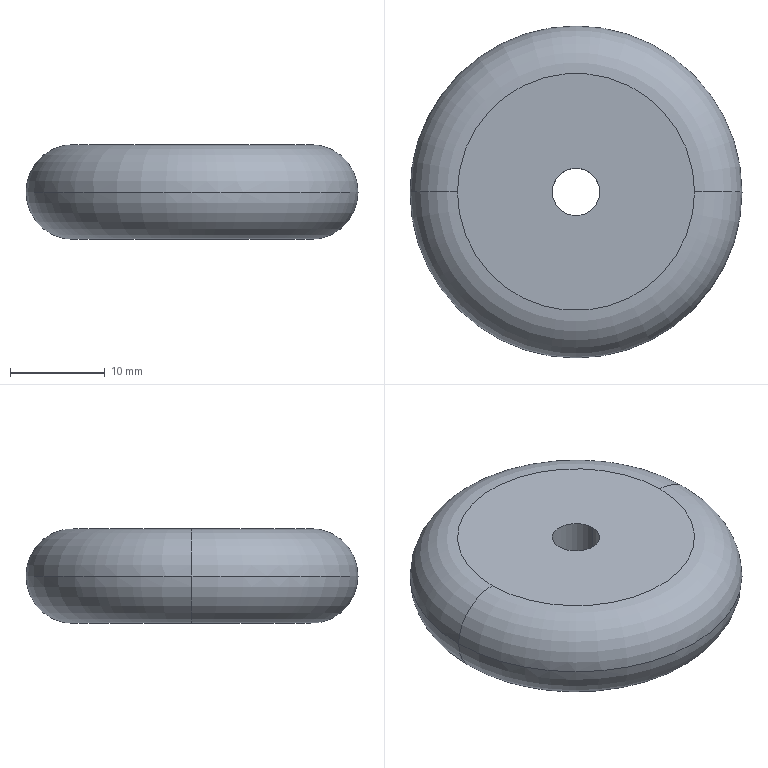Part | SolidWorks | features Extrusion 1, Fillet 1, ICE 1 | 1 solid | 8 faces | box 35 x 35 x 10 mm | volume 8320 mm3 | torus 4 | cylinder 2 | plane 2 | commonest cylinder face diameters 5 x2
STEP:
#1=CARTESIAN_POINT('',(2.5,0.,10.));
#2=VERTEX_POINT('',#1);
#3=CARTESIAN_POINT('',(-2.5,0.,10.));
#4=VERTEX_POINT('',#3);
#5=CARTESIAN_POINT('',(0.,0.,10.));
#6=DIRECTION('',(0.,0.,-1.));
#7=DIRECTION('',(1.,0.,0.));
#8=AXIS2_PLACEMENT_3D('',#5,#6,#7);
#9=CIRCLE('',#8,2.5);
#10=EDGE_CURVE('',#2,#4,#9,.T.);
#11=ORIENTED_EDGE('',*,*,#10,.F.);
#12=CARTESIAN_POINT('',(2.5,0.,0.));
#13=VERTEX_POINT('',#12);
#14=CARTESIAN_POINT('',(2.5,0.,17.071));
#15=DIRECTION('',(0.,0.,-1.));
#16=VECTOR('',#15,1000.);
#17=LINE('',#14,#16);
#18=EDGE_CURVE('',#2,#13,#17,.T.);
#19=ORIENTED_EDGE('',*,*,#18,.T.);
#20=CARTESIAN_POINT('',(-2.5,0.,0.));
#21=VERTEX_POINT('',#20);
#22=CARTESIAN_POINT('',(0.,0.,0.));
#23=DIRECTION('',(0.,0.,-1.));
#24=DIRECTION('',(-1.,0.,0.));
#25=AXIS2_PLACEMENT_3D('',#22,#23,#24);
#26=CIRCLE('',#25,2.5);
#27=EDGE_CURVE('',#13,#21,#26,.T.);
#28=ORIENTED_EDGE('',*,*,#27,.T.);
#29=CARTESIAN_POINT('',(-2.5,0.,17.071));
#30=DIRECTION('',(0.,0.,-1.));
#31=VECTOR('',#30,1000.);
#32=LINE('',#29,#31);
#33=EDGE_CURVE('',#4,#21,#32,.T.);
#34=ORIENTED_EDGE('',*,*,#33,.F.);
#35=EDGE_LOOP('',(#11,#19,#28,#34));
#36=FACE_OUTER_BOUND('',#35,.T.);
#37=CARTESIAN_POINT('',(0.,0.,17.071));
#38=DIRECTION('',(0.,0.,-1.));
#39=DIRECTION('',(-1.,0.,0.));
#40=AXIS2_PLACEMENT_3D('',#37,#38,#39);
#41=CYLINDRICAL_SURFACE('',#40,2.5);
#42=ADVANCED_FACE('',(#36),#41,.F.);
#43=CARTESIAN_POINT('',(-12.5,0.,0.));
#44=VERTEX_POINT('',#43);
#45=CARTESIAN_POINT('',(12.5,0.,0.));
#46=VERTEX_POINT('',#45);
#47=CARTESIAN_POINT('',(0.,0.,0.));
#48=DIRECTION('',(0.,0.,-1.));
#49=DIRECTION('',(1.,0.,0.));
#50=AXIS2_PLACEMENT_3D('',#47,#48,#49);
#51=CIRCLE('',#50,12.5);
#52=EDGE_CURVE('',#44,#46,#51,.T.);
#53=ORIENTED_EDGE('',*,*,#52,.F.);
#54=CARTESIAN_POINT('',(-17.5,0.,5.));
#55=VERTEX_POINT('',#54);
#56=CARTESIAN_POINT('',(-12.5,0.,5.));
#57=DIRECTION('',(0.,1.,0.));
#58=DIRECTION('',(-1.,0.,0.));
#59=AXIS2_PLACEMENT_3D('',#56,#57,#58);
#60=CIRCLE('',#59,5.);
#61=EDGE_CURVE('',#44,#55,#60,.T.);
#62=ORIENTED_EDGE('',*,*,#61,.T.);
#63=CARTESIAN_POINT('',(17.5,0.,5.));
#64=VERTEX_POINT('',#63);
#65=CARTESIAN_POINT('',(0.,0.,5.));
#66=DIRECTION('',(0.,0.,-1.));
#67=DIRECTION('',(1.,0.,0.));
#68=AXIS2_PLACEMENT_3D('',#65,#66,#67);
#69=CIRCLE('',#68,17.5);
#70=EDGE_CURVE('',#55,#64,#69,.T.);
#71=ORIENTED_EDGE('',*,*,#70,.T.);
#72=CARTESIAN_POINT('',(12.5,0.,5.));
#73=DIRECTION('',(0.,-1.,0.));
#74=DIRECTION('',(0.,0.,-1.));
#75=AXIS2_PLACEMENT_3D('',#72,#73,#74);
#76=CIRCLE('',#75,5.);
#77=EDGE_CURVE('',#46,#64,#76,.T.);
#78=ORIENTED_EDGE('',*,*,#77,.F.);
#79=EDGE_LOOP('',(#53,#62,#71,#78));
#80=FACE_OUTER_BOUND('',#79,.T.);
#81=CARTESIAN_POINT('',(0.,0.,5.));
#82=DIRECTION('',(0.,0.,1.));
#83=DIRECTION('',(1.,0.,0.));
#84=AXIS2_PLACEMENT_3D('',#81,#82,#83);
#85=TOROIDAL_SURFACE('',#84,12.5,5.);
#86=ADVANCED_FACE('',(#80),#85,.T.);
#87=ORIENTED_EDGE('',*,*,#70,.F.);
#88=CARTESIAN_POINT('',(-12.5,0.,10.));
#89=VERTEX_POINT('',#88);
#90=CARTESIAN_POINT('',(-12.5,0.,5.));
#91=DIRECTION('',(0.,1.,0.));
#92=DIRECTION('',(-1.,0.,0.));
#93=AXIS2_PLACEMENT_3D('',#90,#91,#92);
#94=CIRCLE('',#93,5.);
#95=EDGE_CURVE('',#55,#89,#94,.T.);
#96=ORIENTED_EDGE('',*,*,#95,.T.);
#97=CARTESIAN_POINT('',(12.5,0.,10.));
#98=VERTEX_POINT('',#97);
#99=CARTESIAN_POINT('',(0.,0.,10.));
#100=DIRECTION('',(0.,0.,1.));
#101=DIRECTION('',(1.,0.,0.));
#102=AXIS2_PLACEMENT_3D('',#99,#100,#101);
#103=CIRCLE('',#102,12.5);
#104=EDGE_CURVE('',#98,#89,#103,.T.);
#105=ORIENTED_EDGE('',*,*,#104,.F.);
#106=CARTESIAN_POINT('',(12.5,0.,5.));
#107=DIRECTION('',(0.,-1.,0.));
#108=DIRECTION('',(0.,0.,-1.));
#109=AXIS2_PLACEMENT_3D('',#106,#107,#108);
#110=CIRCLE('',#109,5.);
#111=EDGE_CURVE('',#64,#98,#110,.T.);
#112=ORIENTED_EDGE('',*,*,#111,.F.);
#113=EDGE_LOOP('',(#87,#96,#105,#112));
#114=FACE_OUTER_BOUND('',#113,.T.);
#115=CARTESIAN_POINT('',(0.,0.,5.));
#116=DIRECTION('',(0.,0.,1.));
#117=DIRECTION('',(1.,0.,0.));
#118=AXIS2_PLACEMENT_3D('',#115,#116,#117);
#119=TOROIDAL_SURFACE('',#118,12.5,5.);
#120=ADVANCED_FACE('',(#114),#119,.T.);
#121=CARTESIAN_POINT('',(0.,0.,10.));
#122=DIRECTION('',(0.,0.,-1.));
#123=DIRECTION('',(1.,0.,0.));
#124=AXIS2_PLACEMENT_3D('',#121,#122,#123);
#125=CIRCLE('',#124,2.5);
#126=EDGE_CURVE('',#4,#2,#125,.T.);
#127=ORIENTED_EDGE('',*,*,#126,.T.);
#128=ORIENTED_EDGE('',*,*,#10,.T.);
#129=EDGE_LOOP('',(#127,#128));
#130=FACE_BOUND('',#129,.T.);
#131=ORIENTED_EDGE('',*,*,#104,.T.);
#132=CARTESIAN_POINT('',(0.,0.,10.));
#133=DIRECTION('',(0.,0.,1.));
#134=DIRECTION('',(1.,0.,0.));
#135=AXIS2_PLACEMENT_3D('',#132,#133,#134);
#136=CIRCLE('',#135,12.5);
#137=EDGE_CURVE('',#89,#98,#136,.T.);
#138=ORIENTED_EDGE('',*,*,#137,.T.);
#139=EDGE_LOOP('',(#131,#138));
#140=FACE_OUTER_BOUND('',#139,.T.);
#141=CARTESIAN_POINT('',(0.,0.,10.));
#142=DIRECTION('',(0.,0.,1.));
#143=DIRECTION('',(1.,0.,0.));
#144=AXIS2_PLACEMENT_3D('',#141,#142,#143);
#145=PLANE('',#144);
#146=ADVANCED_FACE('',(#130,#140),#145,.T.);
#147=CARTESIAN_POINT('',(0.,0.,0.));
#148=DIRECTION('',(0.,0.,-1.));
#149=DIRECTION('',(-1.,0.,0.));
#150=AXIS2_PLACEMENT_3D('',#147,#148,#149);
#151=CIRCLE('',#150,2.5);
#152=EDGE_CURVE('',#21,#13,#151,.T.);
#153=ORIENTED_EDGE('',*,*,#152,.F.);
#154=ORIENTED_EDGE('',*,*,#27,.F.);
#155=EDGE_LOOP('',(#153,#154));
#156=FACE_BOUND('',#155,.T.);
#157=CARTESIAN_POINT('',(0.,0.,0.));
#158=DIRECTION('',(0.,0.,-1.));
#159=DIRECTION('',(1.,0.,0.));
#160=AXIS2_PLACEMENT_3D('',#157,#158,#159);
#161=CIRCLE('',#160,12.5);
#162=EDGE_CURVE('',#46,#44,#161,.T.);
#163=ORIENTED_EDGE('',*,*,#162,.T.);
#164=ORIENTED_EDGE('',*,*,#52,.T.);
#165=EDGE_LOOP('',(#163,#164));
#166=FACE_OUTER_BOUND('',#165,.T.);
#167=CARTESIAN_POINT('',(0.,0.,0.));
#168=DIRECTION('',(0.,0.,1.));
#169=DIRECTION('',(1.,0.,0.));
#170=AXIS2_PLACEMENT_3D('',#167,#168,#169);
#171=PLANE('',#170);
#172=ADVANCED_FACE('',(#156,#166),#171,.F.);
#173=ORIENTED_EDGE('',*,*,#95,.F.);
#174=CARTESIAN_POINT('',(0.,0.,5.));
#175=DIRECTION('',(0.,0.,-1.));
#176=DIRECTION('',(1.,0.,0.));
#177=AXIS2_PLACEMENT_3D('',#174,#175,#176);
#178=CIRCLE('',#177,17.5);
#179=EDGE_CURVE('',#64,#55,#178,.T.);
#180=ORIENTED_EDGE('',*,*,#179,.F.);
#181=ORIENTED_EDGE('',*,*,#111,.T.);
#182=ORIENTED_EDGE('',*,*,#137,.F.);
#183=EDGE_LOOP('',(#173,#180,#181,#182));
#184=FACE_OUTER_BOUND('',#183,.T.);
#185=CARTESIAN_POINT('',(0.,0.,5.));
#186=DIRECTION('',(0.,0.,1.));
#187=DIRECTION('',(1.,0.,0.));
#188=AXIS2_PLACEMENT_3D('',#185,#186,#187);
#189=TOROIDAL_SURFACE('',#188,12.5,5.);
#190=ADVANCED_FACE('',(#184),#189,.T.);
#191=ORIENTED_EDGE('',*,*,#61,.F.);
#192=ORIENTED_EDGE('',*,*,#162,.F.);
#193=ORIENTED_EDGE('',*,*,#77,.T.);
#194=ORIENTED_EDGE('',*,*,#179,.T.);
#195=EDGE_LOOP('',(#191,#192,#193,#194));
#196=FACE_OUTER_BOUND('',#195,.T.);
#197=CARTESIAN_POINT('',(0.,0.,5.));
#198=DIRECTION('',(0.,0.,1.));
#199=DIRECTION('',(1.,0.,0.));
#200=AXIS2_PLACEMENT_3D('',#197,#198,#199);
#201=TOROIDAL_SURFACE('',#200,12.5,5.);
#202=ADVANCED_FACE('',(#196),#201,.T.);
#203=ORIENTED_EDGE('',*,*,#18,.F.);
#204=ORIENTED_EDGE('',*,*,#126,.F.);
#205=ORIENTED_EDGE('',*,*,#33,.T.);
#206=ORIENTED_EDGE('',*,*,#152,.T.);
#207=EDGE_LOOP('',(#203,#204,#205,#206));
#208=FACE_OUTER_BOUND('',#207,.T.);
#209=CARTESIAN_POINT('',(0.,0.,17.071));
#210=DIRECTION('',(0.,0.,-1.));
#211=DIRECTION('',(-1.,0.,0.));
#212=AXIS2_PLACEMENT_3D('',#209,#210,#211);
#213=CYLINDRICAL_SURFACE('',#212,2.5);
#214=ADVANCED_FACE('',(#208),#213,.F.);
#215=CLOSED_SHELL('',(#42,#86,#120,#146,#172,#190,#202,#214));
#216=MANIFOLD_SOLID_BREP('',#215);
#217=CARTESIAN_POINT('',(0.,0.,0.));
#218=DIRECTION('',(0.,0.,1.));
#219=DIRECTION('',(1.,0.,0.));
#220=AXIS2_PLACEMENT_3D('',#217,#218,#219);
#221=(LENGTH_UNIT()NAMED_UNIT(*)SI_UNIT(.MILLI.,.METRE.));
#222=UNCERTAINTY_MEASURE_WITH_UNIT(LENGTH_MEASURE(0.00001),#221,'','');
#223=(NAMED_UNIT(*)PLANE_ANGLE_UNIT()SI_UNIT($,.RADIAN.));
#224=(NAMED_UNIT(*)SI_UNIT($,.STERADIAN.)SOLID_ANGLE_UNIT());
#225=(GEOMETRIC_REPRESENTATION_CONTEXT(3)GLOBAL_UNCERTAINTY_ASSIGNED_CONTEXT((#222))GLOBAL_UNIT_ASSIGNED_CONTEXT((#221,#223,#224))REPRESENTATION_CONTEXT('',''));
#226=ADVANCED_BREP_SHAPE_REPRESENTATION('',(#216,#220),#225);